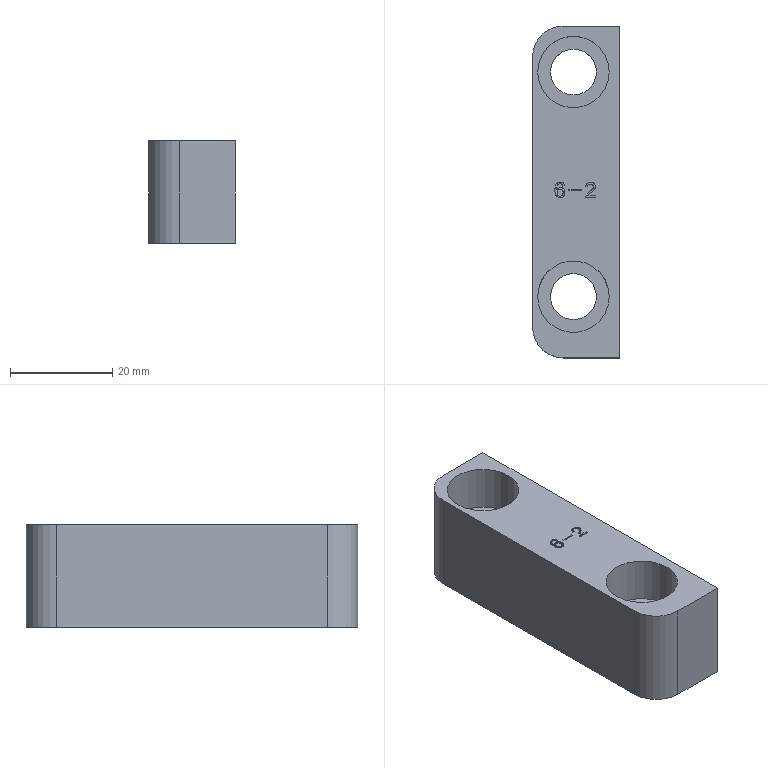Part | STEP file | solid 14 | 1 solid | 33 faces | box 17 x 65 x 20 mm | volume 17619 mm3 | plane 21 | cylinder 6 | other 6 | commonest cylinder face diameters 9 x2 12 x2 14 x2